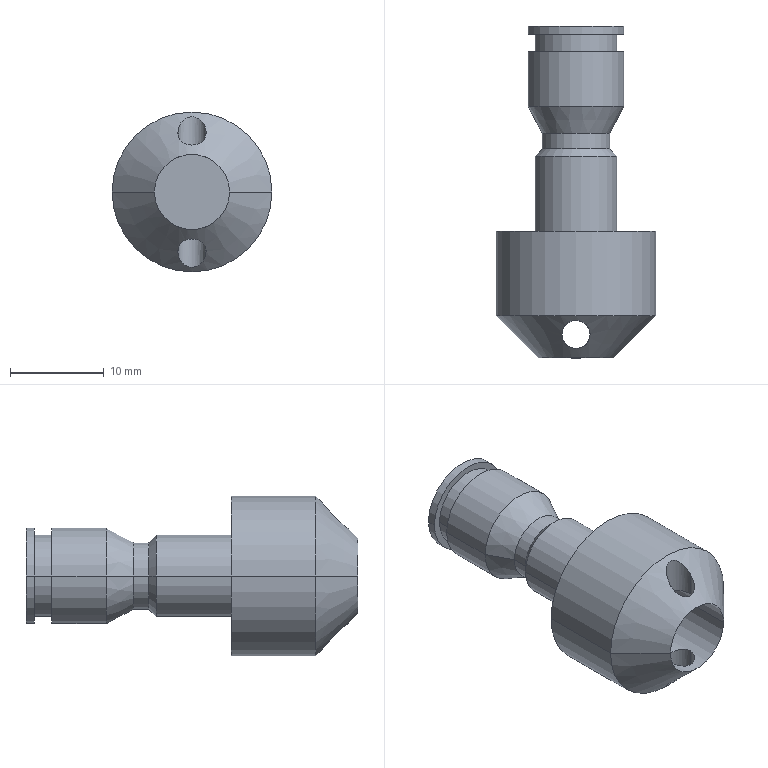Part | SolidWorks | features Cut 1, ICE 1, MirrorPattern 1, RevCut 1, Revolution 1 | 1 solid | 32 faces | box 17 x 35.31 x 17 mm | volume 3384 mm3 | cylinder 20 | cone 6 | plane 6 | commonest cylinder face diameters 3 x4 8.682 x4 10.203 x4 5.5 x2 7.161 x2 8 x2
STEP:
#1=CARTESIAN_POINT('',(-1.5,-17.445,6.325));
#2=VERTEX_POINT('',#1);
#3=CARTESIAN_POINT('',(1.5,-17.445,6.325));
#4=VERTEX_POINT('',#3);
#5=CARTESIAN_POINT('',(-1.5,-17.445,6.325));
#6=CARTESIAN_POINT('',(-1.5,-17.274,6.501));
#7=CARTESIAN_POINT('',(-1.472,-17.107,6.679));
#8=CARTESIAN_POINT('',(-1.356,-16.781,7.035));
#9=CARTESIAN_POINT('',(-1.271,-16.627,7.208));
#10=CARTESIAN_POINT('',(-1.033,-16.342,7.534));
#11=CARTESIAN_POINT('',(-0.8798,-16.211,7.687));
#12=CARTESIAN_POINT('',(-0.5873,-16.06,7.863));
#13=CARTESIAN_POINT('',(-0.4808,-16.019,7.912));
#14=CARTESIAN_POINT('',(-0.2477,-15.961,7.981));
#15=CARTESIAN_POINT('',(-0.1246,-15.945,8.));
#16=CARTESIAN_POINT('',(0.1245,-15.945,8.));
#17=CARTESIAN_POINT('',(0.248,-15.961,7.981));
#18=CARTESIAN_POINT('',(0.4799,-16.019,7.913));
#19=CARTESIAN_POINT('',(0.5882,-16.061,7.863));
#20=CARTESIAN_POINT('',(0.8792,-16.21,7.687));
#21=CARTESIAN_POINT('',(1.033,-16.342,7.534));
#22=CARTESIAN_POINT('',(1.27,-16.626,7.21));
#23=CARTESIAN_POINT('',(1.357,-16.782,7.034));
#24=CARTESIAN_POINT('',(1.471,-17.105,6.681));
#25=CARTESIAN_POINT('',(1.5,-17.272,6.502));
#26=CARTESIAN_POINT('',(1.5,-17.445,6.325));
#27=B_SPLINE_CURVE_WITH_KNOTS('',3,(#5,#6,#7,#8,#9,#10,#11,#12,#13,#14,#15,#16,#17,#18,#19,#20,#21,#22,#23,#24,#25,#26),.UNSPECIFIED.,.F.,.F.,(4,2,2,2,2,2,2,2,2,2,4),(0.0021,0.002839,0.003577,0.004316,0.004685,0.005054,0.005424,0.005793,0.006531,0.00727,0.008009),.UNSPECIFIED.);
#28=EDGE_CURVE('',#2,#4,#27,.T.);
#29=ORIENTED_EDGE('',*,*,#28,.F.);
#30=CARTESIAN_POINT('',(-1.5,-17.445,3.708));
#31=VERTEX_POINT('',#30);
#32=CARTESIAN_POINT('',(-1.5,-17.445,3.483));
#33=DIRECTION('',(0.,0.,-1.));
#34=VECTOR('',#33,1000.);
#35=LINE('',#32,#34);
#36=EDGE_CURVE('',#2,#31,#35,.T.);
#37=ORIENTED_EDGE('',*,*,#36,.T.);
#38=CARTESIAN_POINT('',(1.5,-17.445,3.708));
#39=VERTEX_POINT('',#38);
#40=CARTESIAN_POINT('',(-1.5,-17.445,3.708));
#41=CARTESIAN_POINT('',(-1.5,-17.248,3.708));
#42=CARTESIAN_POINT('',(-1.46,-17.049,3.725));
#43=CARTESIAN_POINT('',(-1.347,-16.777,3.767));
#44=CARTESIAN_POINT('',(-1.3,-16.69,3.783));
#45=CARTESIAN_POINT('',(-1.191,-16.529,3.819));
#46=CARTESIAN_POINT('',(-1.13,-16.453,3.838));
#47=CARTESIAN_POINT('',(-0.9215,-16.245,3.895));
#48=CARTESIAN_POINT('',(-0.7581,-16.136,3.932));
#49=CARTESIAN_POINT('',(-0.4854,-16.022,3.971));
#50=CARTESIAN_POINT('',(-0.3917,-15.994,3.982));
#51=CARTESIAN_POINT('',(-0.1986,-15.955,3.996));
#52=CARTESIAN_POINT('',(-0.09814,-15.945,4.));
#53=CARTESIAN_POINT('',(0.1984,-15.945,4.));
#54=CARTESIAN_POINT('',(0.3972,-15.985,3.984));
#55=CARTESIAN_POINT('',(0.7586,-16.136,3.932));
#56=CARTESIAN_POINT('',(0.924,-16.248,3.894));
#57=CARTESIAN_POINT('',(1.13,-16.454,3.838));
#58=CARTESIAN_POINT('',(1.193,-16.53,3.818));
#59=CARTESIAN_POINT('',(1.301,-16.692,3.783));
#60=CARTESIAN_POINT('',(1.347,-16.778,3.767));
#61=CARTESIAN_POINT('',(1.461,-17.051,3.725));
#62=CARTESIAN_POINT('',(1.5,-17.245,3.708));
#63=CARTESIAN_POINT('',(1.5,-17.445,3.708));
#64=B_SPLINE_CURVE_WITH_KNOTS('',3,(#40,#41,#42,#43,#44,#45,#46,#47,#48,#49,#50,#51,#52,#53,#54,#55,#56,#57,#58,#59,#60,#61,#62,#63),.UNSPECIFIED.,.F.,.F.,(4,2,2,2,2,2,2,2,2,2,2,4),(0.004733,0.005325,0.00562,0.005916,0.006508,0.006803,0.007099,0.007691,0.008282,0.008578,0.008874,0.009465),.UNSPECIFIED.);
#65=EDGE_CURVE('',#31,#39,#64,.T.);
#66=ORIENTED_EDGE('',*,*,#65,.T.);
#67=CARTESIAN_POINT('',(1.5,-17.445,3.483));
#68=DIRECTION('',(0.,0.,-1.));
#69=VECTOR('',#68,1000.);
#70=LINE('',#67,#69);
#71=EDGE_CURVE('',#4,#39,#70,.T.);
#72=ORIENTED_EDGE('',*,*,#71,.F.);
#73=EDGE_LOOP('',(#29,#37,#66,#72));
#74=FACE_OUTER_BOUND('',#73,.T.);
#75=CARTESIAN_POINT('',(0.,-17.445,3.483));
#76=DIRECTION('',(0.,0.,-1.));
#77=DIRECTION('',(1.,0.,0.));
#78=AXIS2_PLACEMENT_3D('',#75,#76,#77);
#79=CYLINDRICAL_SURFACE('',#78,1.5);
#80=ADVANCED_FACE('',(#74),#79,.F.);
#81=CARTESIAN_POINT('',(-1.5,-17.445,-6.325));
#82=VERTEX_POINT('',#81);
#83=CARTESIAN_POINT('',(1.5,-17.445,-6.325));
#84=VERTEX_POINT('',#83);
#85=CARTESIAN_POINT('',(-1.5,-17.445,-6.325));
#86=CARTESIAN_POINT('',(-1.5,-17.607,-6.158));
#87=CARTESIAN_POINT('',(-1.474,-17.773,-5.994));
#88=CARTESIAN_POINT('',(-1.362,-18.098,-5.687));
#89=CARTESIAN_POINT('',(-1.273,-18.261,-5.54));
#90=CARTESIAN_POINT('',(-1.024,-18.558,-5.29));
#91=CARTESIAN_POINT('',(-0.8599,-18.694,-5.184));
#92=CARTESIAN_POINT('',(-0.5617,-18.84,-5.075));
#93=CARTESIAN_POINT('',(-0.4548,-18.879,-5.047));
#94=CARTESIAN_POINT('',(-0.2332,-18.931,-5.01));
#95=CARTESIAN_POINT('',(-0.1157,-18.945,-5.));
#96=CARTESIAN_POINT('',(0.1157,-18.945,-5.));
#97=CARTESIAN_POINT('',(0.2323,-18.931,-5.009));
#98=CARTESIAN_POINT('',(0.4559,-18.879,-5.047));
#99=CARTESIAN_POINT('',(0.562,-18.84,-5.075));
#100=CARTESIAN_POINT('',(0.8615,-18.693,-5.184));
#101=CARTESIAN_POINT('',(1.025,-18.557,-5.291));
#102=CARTESIAN_POINT('',(1.274,-18.26,-5.541));
#103=CARTESIAN_POINT('',(1.362,-18.096,-5.688));
#104=CARTESIAN_POINT('',(1.474,-17.772,-5.995));
#105=CARTESIAN_POINT('',(1.5,-17.606,-6.159));
#106=CARTESIAN_POINT('',(1.5,-17.445,-6.325));
#107=B_SPLINE_CURVE_WITH_KNOTS('',3,(#85,#86,#87,#88,#89,#90,#91,#92,#93,#94,#95,#96,#97,#98,#99,#100,#101,#102,#103,#104,#105,#106),.UNSPECIFIED.,.F.,.F.,(4,2,2,2,2,2,2,2,2,2,4),(0.01111,0.0118,0.01249,0.01319,0.01353,0.01388,0.01422,0.01457,0.01526,0.01595,0.01664),.UNSPECIFIED.);
#108=EDGE_CURVE('',#82,#84,#107,.T.);
#109=ORIENTED_EDGE('',*,*,#108,.F.);
#110=CARTESIAN_POINT('',(-1.5,-17.445,-3.708));
#111=VERTEX_POINT('',#110);
#112=CARTESIAN_POINT('',(-1.5,-17.445,-3.483));
#113=DIRECTION('',(0.,0.,1.));
#114=VECTOR('',#113,1000.);
#115=LINE('',#112,#114);
#116=EDGE_CURVE('',#82,#111,#115,.T.);
#117=ORIENTED_EDGE('',*,*,#116,.T.);
#118=CARTESIAN_POINT('',(1.5,-17.445,-3.708));
#119=VERTEX_POINT('',#118);
#120=CARTESIAN_POINT('',(-1.5,-17.445,-3.708));
#121=CARTESIAN_POINT('',(-1.5,-17.642,-3.708));
#122=CARTESIAN_POINT('',(-1.46,-17.841,-3.725));
#123=CARTESIAN_POINT('',(-1.347,-18.113,-3.767));
#124=CARTESIAN_POINT('',(-1.3,-18.2,-3.783));
#125=CARTESIAN_POINT('',(-1.191,-18.362,-3.819));
#126=CARTESIAN_POINT('',(-1.13,-18.437,-3.838));
#127=CARTESIAN_POINT('',(-0.9215,-18.645,-3.895));
#128=CARTESIAN_POINT('',(-0.7581,-18.754,-3.932));
#129=CARTESIAN_POINT('',(-0.4854,-18.868,-3.971));
#130=CARTESIAN_POINT('',(-0.3917,-18.896,-3.982));
#131=CARTESIAN_POINT('',(-0.1986,-18.935,-3.996));
#132=CARTESIAN_POINT('',(-0.09814,-18.945,-4.));
#133=CARTESIAN_POINT('',(0.1984,-18.945,-4.));
#134=CARTESIAN_POINT('',(0.3972,-18.905,-3.984));
#135=CARTESIAN_POINT('',(0.7586,-18.754,-3.932));
#136=CARTESIAN_POINT('',(0.924,-18.643,-3.894));
#137=CARTESIAN_POINT('',(1.13,-18.436,-3.838));
#138=CARTESIAN_POINT('',(1.193,-18.36,-3.818));
#139=CARTESIAN_POINT('',(1.301,-18.198,-3.783));
#140=CARTESIAN_POINT('',(1.347,-18.112,-3.767));
#141=CARTESIAN_POINT('',(1.461,-17.839,-3.725));
#142=CARTESIAN_POINT('',(1.5,-17.645,-3.708));
#143=CARTESIAN_POINT('',(1.5,-17.445,-3.708));
#144=B_SPLINE_CURVE_WITH_KNOTS('',3,(#120,#121,#122,#123,#124,#125,#126,#127,#128,#129,#130,#131,#132,#133,#134,#135,#136,#137,#138,#139,#140,#141,#142,#143),.UNSPECIFIED.,.F.,.F.,(4,2,2,2,2,2,2,2,2,2,2,4),(0.004733,0.005325,0.00562,0.005916,0.006508,0.006803,0.007099,0.007691,0.008282,0.008578,0.008874,0.009465),.UNSPECIFIED.);
#145=EDGE_CURVE('',#111,#119,#144,.T.);
#146=ORIENTED_EDGE('',*,*,#145,.T.);
#147=CARTESIAN_POINT('',(1.5,-17.445,-3.483));
#148=DIRECTION('',(0.,0.,1.));
#149=VECTOR('',#148,1000.);
#150=LINE('',#147,#149);
#151=EDGE_CURVE('',#84,#119,#150,.T.);
#152=ORIENTED_EDGE('',*,*,#151,.F.);
#153=EDGE_LOOP('',(#109,#117,#146,#152));
#154=FACE_OUTER_BOUND('',#153,.T.);
#155=CARTESIAN_POINT('',(0.,-17.445,-3.483));
#156=DIRECTION('',(0.,0.,1.));
#157=DIRECTION('',(1.,0.,0.));
#158=AXIS2_PLACEMENT_3D('',#155,#156,#157);
#159=CYLINDRICAL_SURFACE('',#158,1.5);
#160=ADVANCED_FACE('',(#154),#159,.F.);
#161=CARTESIAN_POINT('',(2.75,11.365,0.));
#162=VERTEX_POINT('',#161);
#163=CARTESIAN_POINT('',(-2.75,11.365,0.));
#164=VERTEX_POINT('',#163);
#165=CARTESIAN_POINT('',(0.,11.365,0.));
#166=DIRECTION('',(0.,1.,0.));
#167=DIRECTION('',(-1.,0.,0.));
#168=AXIS2_PLACEMENT_3D('',#165,#166,#167);
#169=CIRCLE('',#168,2.75);
#170=EDGE_CURVE('',#162,#164,#169,.T.);
#171=ORIENTED_EDGE('',*,*,#170,.F.);
#172=CARTESIAN_POINT('',(2.75,15.365,0.));
#173=VERTEX_POINT('',#172);
#174=CARTESIAN_POINT('',(2.75,11.365,0.));
#175=DIRECTION('',(0.,1.,0.));
#176=VECTOR('',#175,1000.);
#177=LINE('',#174,#176);
#178=EDGE_CURVE('',#162,#173,#177,.T.);
#179=ORIENTED_EDGE('',*,*,#178,.T.);
#180=CARTESIAN_POINT('',(-2.75,15.365,0.));
#181=VERTEX_POINT('',#180);
#182=CARTESIAN_POINT('',(0.,15.365,0.));
#183=DIRECTION('',(0.,1.,0.));
#184=DIRECTION('',(-1.,0.,0.));
#185=AXIS2_PLACEMENT_3D('',#182,#183,#184);
#186=CIRCLE('',#185,2.75);
#187=EDGE_CURVE('',#173,#181,#186,.T.);
#188=ORIENTED_EDGE('',*,*,#187,.T.);
#189=CARTESIAN_POINT('',(-2.75,11.365,0.));
#190=DIRECTION('',(0.,1.,0.));
#191=VECTOR('',#190,1000.);
#192=LINE('',#189,#191);
#193=EDGE_CURVE('',#164,#181,#192,.T.);
#194=ORIENTED_EDGE('',*,*,#193,.F.);
#195=EDGE_LOOP('',(#171,#179,#188,#194));
#196=FACE_OUTER_BOUND('',#195,.T.);
#197=CARTESIAN_POINT('',(0.,11.365,0.));
#198=DIRECTION('',(0.,1.,0.));
#199=DIRECTION('',(-1.,0.,0.));
#200=AXIS2_PLACEMENT_3D('',#197,#198,#199);
#201=CYLINDRICAL_SURFACE('',#200,2.75);
#202=ADVANCED_FACE('',(#196),#201,.F.);
#203=CARTESIAN_POINT('',(-8.5,-15.445,0.));
#204=VERTEX_POINT('',#203);
#205=CARTESIAN_POINT('',(8.5,-15.445,0.));
#206=VERTEX_POINT('',#205);
#207=CARTESIAN_POINT('',(0.,-15.445,0.));
#208=DIRECTION('',(0.,1.,0.));
#209=DIRECTION('',(-1.,0.,0.));
#210=AXIS2_PLACEMENT_3D('',#207,#208,#209);
#211=CIRCLE('',#210,8.5);
#212=EDGE_CURVE('',#204,#206,#211,.T.);
#213=ORIENTED_EDGE('',*,*,#212,.T.);
#214=CARTESIAN_POINT('',(8.5,-6.487,0.));
#215=VERTEX_POINT('',#214);
#216=CARTESIAN_POINT('',(8.5,12.634,0.));
#217=DIRECTION('',(0.,1.,0.));
#218=VECTOR('',#217,1000.);
#219=LINE('',#216,#218);
#220=EDGE_CURVE('',#206,#215,#219,.T.);
#221=ORIENTED_EDGE('',*,*,#220,.T.);
#222=CARTESIAN_POINT('',(-8.5,-6.487,0.));
#223=VERTEX_POINT('',#222);
#224=CARTESIAN_POINT('',(0.,-6.487,0.));
#225=DIRECTION('',(0.,1.,0.));
#226=DIRECTION('',(-1.,0.,0.));
#227=AXIS2_PLACEMENT_3D('',#224,#225,#226);
#228=CIRCLE('',#227,8.5);
#229=EDGE_CURVE('',#223,#215,#228,.T.);
#230=ORIENTED_EDGE('',*,*,#229,.F.);
#231=CARTESIAN_POINT('',(-8.5,12.634,0.));
#232=DIRECTION('',(0.,1.,0.));
#233=VECTOR('',#232,1000.);
#234=LINE('',#231,#233);
#235=EDGE_CURVE('',#204,#223,#234,.T.);
#236=ORIENTED_EDGE('',*,*,#235,.F.);
#237=EDGE_LOOP('',(#213,#221,#230,#236));
#238=FACE_OUTER_BOUND('',#237,.T.);
#239=CARTESIAN_POINT('',(0.,12.634,0.));
#240=DIRECTION('',(0.,1.,0.));
#241=DIRECTION('',(-1.,0.,0.));
#242=AXIS2_PLACEMENT_3D('',#239,#240,#241);
#243=CYLINDRICAL_SURFACE('',#242,8.5);
#244=ADVANCED_FACE('',(#238),#243,.T.);
#245=CARTESIAN_POINT('',(-4.341,-6.487,0.));
#246=VERTEX_POINT('',#245);
#247=CARTESIAN_POINT('',(4.341,-6.487,0.));
#248=VERTEX_POINT('',#247);
#249=CARTESIAN_POINT('',(0.,-6.487,0.));
#250=DIRECTION('',(0.,1.,0.));
#251=DIRECTION('',(-1.,0.,0.));
#252=AXIS2_PLACEMENT_3D('',#249,#250,#251);
#253=CIRCLE('',#252,4.341);
#254=EDGE_CURVE('',#246,#248,#253,.T.);
#255=ORIENTED_EDGE('',*,*,#254,.T.);
#256=CARTESIAN_POINT('',(4.341,1.533,0.));
#257=VERTEX_POINT('',#256);
#258=CARTESIAN_POINT('',(4.341,12.634,0.));
#259=DIRECTION('',(0.,1.,0.));
#260=VECTOR('',#259,1000.);
#261=LINE('',#258,#260);
#262=EDGE_CURVE('',#248,#257,#261,.T.);
#263=ORIENTED_EDGE('',*,*,#262,.T.);
#264=CARTESIAN_POINT('',(-4.341,1.533,0.));
#265=VERTEX_POINT('',#264);
#266=CARTESIAN_POINT('',(0.,1.533,0.));
#267=DIRECTION('',(0.,1.,0.));
#268=DIRECTION('',(-1.,0.,0.));
#269=AXIS2_PLACEMENT_3D('',#266,#267,#268);
#270=CIRCLE('',#269,4.341);
#271=EDGE_CURVE('',#265,#257,#270,.T.);
#272=ORIENTED_EDGE('',*,*,#271,.F.);
#273=CARTESIAN_POINT('',(-4.341,12.634,0.));
#274=DIRECTION('',(0.,1.,0.));
#275=VECTOR('',#274,1000.);
#276=LINE('',#273,#275);
#277=EDGE_CURVE('',#246,#265,#276,.T.);
#278=ORIENTED_EDGE('',*,*,#277,.F.);
#279=EDGE_LOOP('',(#255,#263,#272,#278));
#280=FACE_OUTER_BOUND('',#279,.T.);
#281=CARTESIAN_POINT('',(0.,12.634,0.));
#282=DIRECTION('',(0.,1.,0.));
#283=DIRECTION('',(-1.,0.,0.));
#284=AXIS2_PLACEMENT_3D('',#281,#282,#283);
#285=CYLINDRICAL_SURFACE('',#284,4.341);
#286=ADVANCED_FACE('',(#280),#285,.T.);
#287=CARTESIAN_POINT('',(-3.581,2.293,0.));
#288=VERTEX_POINT('',#287);
#289=CARTESIAN_POINT('',(3.581,2.293,0.));
#290=VERTEX_POINT('',#289);
#291=CARTESIAN_POINT('',(0.,2.293,0.));
#292=DIRECTION('',(0.,1.,0.));
#293=DIRECTION('',(-1.,0.,0.));
#294=AXIS2_PLACEMENT_3D('',#291,#292,#293);
#295=CIRCLE('',#294,3.581);
#296=EDGE_CURVE('',#288,#290,#295,.T.);
#297=ORIENTED_EDGE('',*,*,#296,.F.);
#298=CARTESIAN_POINT('',(-3.581,2.293,0.));
#299=DIRECTION('',(-0.7071,-0.7071,0.));
#300=VECTOR('',#299,1000.);
#301=LINE('',#298,#300);
#302=EDGE_CURVE('',#288,#265,#301,.T.);
#303=ORIENTED_EDGE('',*,*,#302,.T.);
#304=ORIENTED_EDGE('',*,*,#271,.T.);
#305=CARTESIAN_POINT('',(3.581,2.293,0.));
#306=DIRECTION('',(0.7071,-0.7071,0.));
#307=VECTOR('',#306,1000.);
#308=LINE('',#305,#307);
#309=EDGE_CURVE('',#290,#257,#308,.T.);
#310=ORIENTED_EDGE('',*,*,#309,.F.);
#311=EDGE_LOOP('',(#297,#303,#304,#310));
#312=FACE_OUTER_BOUND('',#311,.T.);
#313=CARTESIAN_POINT('',(0.,2.293,0.));
#314=DIRECTION('',(0.,-1.,0.));
#315=DIRECTION('',(1.,0.,0.));
#316=AXIS2_PLACEMENT_3D('',#313,#314,#315);
#317=CONICAL_SURFACE('',#316,3.581,0.7854);
#318=ADVANCED_FACE('',(#312),#317,.T.);
#319=ORIENTED_EDGE('',*,*,#296,.T.);
#320=CARTESIAN_POINT('',(3.581,3.948,0.));
#321=VERTEX_POINT('',#320);
#322=CARTESIAN_POINT('',(3.581,12.634,0.));
#323=DIRECTION('',(0.,1.,0.));
#324=VECTOR('',#323,1000.);
#325=LINE('',#322,#324);
#326=EDGE_CURVE('',#290,#321,#325,.T.);
#327=ORIENTED_EDGE('',*,*,#326,.T.);
#328=CARTESIAN_POINT('',(-3.581,3.948,0.));
#329=VERTEX_POINT('',#328);
#330=CARTESIAN_POINT('',(0.,3.948,0.));
#331=DIRECTION('',(0.,1.,0.));
#332=DIRECTION('',(-1.,0.,0.));
#333=AXIS2_PLACEMENT_3D('',#330,#331,#332);
#334=CIRCLE('',#333,3.581);
#335=EDGE_CURVE('',#329,#321,#334,.T.);
#336=ORIENTED_EDGE('',*,*,#335,.F.);
#337=CARTESIAN_POINT('',(-3.581,12.634,0.));
#338=DIRECTION('',(0.,1.,0.));
#339=VECTOR('',#338,1000.);
#340=LINE('',#337,#339);
#341=EDGE_CURVE('',#288,#329,#340,.T.);
#342=ORIENTED_EDGE('',*,*,#341,.F.);
#343=EDGE_LOOP('',(#319,#327,#336,#342));
#344=FACE_OUTER_BOUND('',#343,.T.);
#345=CARTESIAN_POINT('',(0.,12.634,0.));
#346=DIRECTION('',(0.,1.,0.));
#347=DIRECTION('',(-1.,0.,0.));
#348=AXIS2_PLACEMENT_3D('',#345,#346,#347);
#349=CYLINDRICAL_SURFACE('',#348,3.581);
#350=ADVANCED_FACE('',(#344),#349,.T.);
#351=ORIENTED_EDGE('',*,*,#335,.T.);
#352=CARTESIAN_POINT('',(5.102,6.827,0.));
#353=VERTEX_POINT('',#352);
#354=CARTESIAN_POINT('',(5.102,6.827,0.));
#355=DIRECTION('',(0.4672,0.8842,0.));
#356=VECTOR('',#355,1000.);
#357=LINE('',#354,#356);
#358=EDGE_CURVE('',#321,#353,#357,.T.);
#359=ORIENTED_EDGE('',*,*,#358,.T.);
#360=CARTESIAN_POINT('',(-5.102,6.827,0.));
#361=VERTEX_POINT('',#360);
#362=CARTESIAN_POINT('',(0.,6.827,0.));
#363=DIRECTION('',(0.,1.,0.));
#364=DIRECTION('',(-1.,0.,0.));
#365=AXIS2_PLACEMENT_3D('',#362,#363,#364);
#366=CIRCLE('',#365,5.102);
#367=EDGE_CURVE('',#361,#353,#366,.T.);
#368=ORIENTED_EDGE('',*,*,#367,.F.);
#369=CARTESIAN_POINT('',(-5.102,6.827,0.));
#370=DIRECTION('',(-0.4672,0.8842,0.));
#371=VECTOR('',#370,1000.);
#372=LINE('',#369,#371);
#373=EDGE_CURVE('',#329,#361,#372,.T.);
#374=ORIENTED_EDGE('',*,*,#373,.F.);
#375=EDGE_LOOP('',(#351,#359,#368,#374));
#376=FACE_OUTER_BOUND('',#375,.T.);
#377=CARTESIAN_POINT('',(0.,6.827,0.));
#378=DIRECTION('',(0.,1.,0.));
#379=DIRECTION('',(-1.,0.,0.));
#380=AXIS2_PLACEMENT_3D('',#377,#378,#379);
#381=CONICAL_SURFACE('',#380,5.102,0.4861);
#382=ADVANCED_FACE('',(#376),#381,.T.);
#383=ORIENTED_EDGE('',*,*,#367,.T.);
#384=CARTESIAN_POINT('',(5.102,12.634,0.));
#385=VERTEX_POINT('',#384);
#386=CARTESIAN_POINT('',(5.102,12.634,0.));
#387=DIRECTION('',(0.,1.,0.));
#388=VECTOR('',#387,1000.);
#389=LINE('',#386,#388);
#390=EDGE_CURVE('',#353,#385,#389,.T.);
#391=ORIENTED_EDGE('',*,*,#390,.T.);
#392=CARTESIAN_POINT('',(-5.102,12.634,0.));
#393=VERTEX_POINT('',#392);
#394=CARTESIAN_POINT('',(0.,12.634,0.));
#395=DIRECTION('',(0.,1.,0.));
#396=DIRECTION('',(-1.,0.,0.));
#397=AXIS2_PLACEMENT_3D('',#394,#395,#396);
#398=CIRCLE('',#397,5.102);
#399=EDGE_CURVE('',#393,#385,#398,.T.);
#400=ORIENTED_EDGE('',*,*,#399,.F.);
#401=CARTESIAN_POINT('',(-5.102,12.634,0.));
#402=DIRECTION('',(0.,1.,0.));
#403=VECTOR('',#402,1000.);
#404=LINE('',#401,#403);
#405=EDGE_CURVE('',#361,#393,#404,.T.);
#406=ORIENTED_EDGE('',*,*,#405,.F.);
#407=EDGE_LOOP('',(#383,#391,#400,#406));
#408=FACE_OUTER_BOUND('',#407,.T.);
#409=CARTESIAN_POINT('',(0.,12.634,0.));
#410=DIRECTION('',(0.,1.,0.));
#411=DIRECTION('',(-1.,0.,0.));
#412=AXIS2_PLACEMENT_3D('',#409,#410,#411);
#413=CYLINDRICAL_SURFACE('',#412,5.102);
#414=ADVANCED_FACE('',(#408),#413,.T.);
#415=CARTESIAN_POINT('',(-4.341,12.634,0.));
#416=VERTEX_POINT('',#415);
#417=CARTESIAN_POINT('',(4.341,12.634,0.));
#418=VERTEX_POINT('',#417);
#419=CARTESIAN_POINT('',(0.,12.634,0.));
#420=DIRECTION('',(0.,1.,0.));
#421=DIRECTION('',(-1.,0.,0.));
#422=AXIS2_PLACEMENT_3D('',#419,#420,#421);
#423=CIRCLE('',#422,4.341);
#424=EDGE_CURVE('',#416,#418,#423,.T.);
#425=ORIENTED_EDGE('',*,*,#424,.T.);
#426=CARTESIAN_POINT('',(4.341,14.471,0.));
#427=VERTEX_POINT('',#426);
#428=CARTESIAN_POINT('',(4.341,12.634,0.));
#429=DIRECTION('',(0.,1.,0.));
#430=VECTOR('',#429,1000.);
#431=LINE('',#428,#430);
#432=EDGE_CURVE('',#418,#427,#431,.T.);
#433=ORIENTED_EDGE('',*,*,#432,.T.);
#434=CARTESIAN_POINT('',(-4.341,14.471,0.));
#435=VERTEX_POINT('',#434);
#436=CARTESIAN_POINT('',(0.,14.471,0.));
#437=DIRECTION('',(0.,1.,0.));
#438=DIRECTION('',(-1.,0.,0.));
#439=AXIS2_PLACEMENT_3D('',#436,#437,#438);
#440=CIRCLE('',#439,4.341);
#441=EDGE_CURVE('',#435,#427,#440,.T.);
#442=ORIENTED_EDGE('',*,*,#441,.F.);
#443=CARTESIAN_POINT('',(-4.341,12.634,0.));
#444=DIRECTION('',(0.,1.,0.));
#445=VECTOR('',#444,1000.);
#446=LINE('',#443,#445);
#447=EDGE_CURVE('',#416,#435,#446,.T.);
#448=ORIENTED_EDGE('',*,*,#447,.F.);
#449=EDGE_LOOP('',(#425,#433,#442,#448));
#450=FACE_OUTER_BOUND('',#449,.T.);
#451=CARTESIAN_POINT('',(0.,12.634,0.));
#452=DIRECTION('',(0.,1.,0.));
#453=DIRECTION('',(-1.,0.,0.));
#454=AXIS2_PLACEMENT_3D('',#451,#452,#453);
#455=CYLINDRICAL_SURFACE('',#454,4.341);
#456=ADVANCED_FACE('',(#450),#455,.T.);
#457=CARTESIAN_POINT('',(-5.102,14.471,0.));
#458=VERTEX_POINT('',#457);
#459=CARTESIAN_POINT('',(5.102,14.471,0.));
#460=VERTEX_POINT('',#459);
#461=CARTESIAN_POINT('',(0.,14.471,0.));
#462=DIRECTION('',(0.,1.,0.));
#463=DIRECTION('',(-1.,0.,0.));
#464=AXIS2_PLACEMENT_3D('',#461,#462,#463);
#465=CIRCLE('',#464,5.102);
#466=EDGE_CURVE('',#458,#460,#465,.T.);
#467=ORIENTED_EDGE('',*,*,#466,.T.);
#468=CARTESIAN_POINT('',(5.102,15.365,0.));
#469=VERTEX_POINT('',#468);
#470=CARTESIAN_POINT('',(5.102,12.634,0.));
#471=DIRECTION('',(0.,1.,0.));
#472=VECTOR('',#471,1000.);
#473=LINE('',#470,#472);
#474=EDGE_CURVE('',#460,#469,#473,.T.);
#475=ORIENTED_EDGE('',*,*,#474,.T.);
#476=CARTESIAN_POINT('',(-5.102,15.365,0.));
#477=VERTEX_POINT('',#476);
#478=CARTESIAN_POINT('',(0.,15.365,0.));
#479=DIRECTION('',(0.,1.,0.));
#480=DIRECTION('',(-1.,0.,0.));
#481=AXIS2_PLACEMENT_3D('',#478,#479,#480);
#482=CIRCLE('',#481,5.102);
#483=EDGE_CURVE('',#477,#469,#482,.T.);
#484=ORIENTED_EDGE('',*,*,#483,.F.);
#485=CARTESIAN_POINT('',(-5.102,12.634,0.));
#486=DIRECTION('',(0.,1.,0.));
#487=VECTOR('',#486,1000.);
#488=LINE('',#485,#487);
#489=EDGE_CURVE('',#458,#477,#488,.T.);
#490=ORIENTED_EDGE('',*,*,#489,.F.);
#491=EDGE_LOOP('',(#467,#475,#484,#490));
#492=FACE_OUTER_BOUND('',#491,.T.);
#493=CARTESIAN_POINT('',(0.,12.634,0.));
#494=DIRECTION('',(0.,1.,0.));
#495=DIRECTION('',(-1.,0.,0.));
#496=AXIS2_PLACEMENT_3D('',#493,#494,#495);
#497=CYLINDRICAL_SURFACE('',#496,5.102);
#498=ADVANCED_FACE('',(#492),#497,.T.);
#499=CARTESIAN_POINT('',(1.5,-17.445,-3.708));
#500=CARTESIAN_POINT('',(1.5,-17.345,-3.708));
#501=CARTESIAN_POINT('',(1.49,-17.247,-3.712));
#502=CARTESIAN_POINT('',(1.451,-17.054,-3.727));
#503=CARTESIAN_POINT('',(1.422,-16.958,-3.739));
#504=CARTESIAN_POINT('',(1.309,-16.686,-3.781));
#505=CARTESIAN_POINT('',(1.198,-16.521,-3.819));
#506=CARTESIAN_POINT('',(0.9235,-16.247,-3.895));
#507=CARTESIAN_POINT('',(0.7577,-16.136,-3.932));
#508=CARTESIAN_POINT('',(0.4873,-16.023,-3.971));
#509=CARTESIAN_POINT('',(0.3918,-15.994,-3.982));
#510=CARTESIAN_POINT('',(0.1976,-15.955,-3.996));
#511=CARTESIAN_POINT('',(0.09965,-15.945,-4.));
#512=CARTESIAN_POINT('',(-0.09818,-15.945,-4.));
#513=CARTESIAN_POINT('',(-0.1986,-15.955,-3.996));
#514=CARTESIAN_POINT('',(-0.3918,-15.994,-3.982));
#515=CARTESIAN_POINT('',(-0.4859,-16.022,-3.971));
#516=CARTESIAN_POINT('',(-0.6688,-16.099,-3.945));
#517=CARTESIAN_POINT('',(-0.7549,-16.145,-3.929));
#518=CARTESIAN_POINT('',(-0.9165,-16.254,-3.894));
#519=CARTESIAN_POINT('',(-0.9928,-16.316,-3.875));
#520=CARTESIAN_POINT('',(-1.13,-16.454,-3.838));
#521=CARTESIAN_POINT('',(-1.192,-16.529,-3.819));
#522=CARTESIAN_POINT('',(-1.3,-16.691,-3.783));
#523=CARTESIAN_POINT('',(-1.347,-16.779,-3.766));
#524=CARTESIAN_POINT('',(-1.46,-17.049,-3.725));
#525=CARTESIAN_POINT('',(-1.5,-17.248,-3.708));
#526=CARTESIAN_POINT('',(-1.5,-17.445,-3.708));
#527=B_SPLINE_CURVE_WITH_KNOTS('',3,(#499,#500,#501,#502,#503,#504,#505,#506,#507,#508,#509,#510,#511,#512,#513,#514,#515,#516,#517,#518,#519,#520,#521,#522,#523,#524,#525,#526),.UNSPECIFIED.,.F.,.F.,(4,2,2,2,2,2,2,2,2,2,2,2,2,4),(0.,0.0002958,0.0005916,0.001183,0.001775,0.002071,0.002367,0.002662,0.002958,0.003254,0.00355,0.003846,0.004142,0.004733),.UNSPECIFIED.);
#528=EDGE_CURVE('',#119,#111,#527,.T.);
#529=ORIENTED_EDGE('',*,*,#528,.F.);
#530=ORIENTED_EDGE('',*,*,#145,.F.);
#531=EDGE_LOOP('',(#529,#530));
#532=FACE_BOUND('',#531,.T.);
#533=CARTESIAN_POINT('',(-4.,-9.945,0.));
#534=VERTEX_POINT('',#533);
#535=CARTESIAN_POINT('',(4.,-9.945,0.));
#536=VERTEX_POINT('',#535);
#537=CARTESIAN_POINT('',(0.,-9.945,0.));
#538=DIRECTION('',(0.,-1.,0.));
#539=DIRECTION('',(1.,0.,0.));
#540=AXIS2_PLACEMENT_3D('',#537,#538,#539);
#541=CIRCLE('',#540,4.);
#542=EDGE_CURVE('',#534,#536,#541,.T.);
#543=ORIENTED_EDGE('',*,*,#542,.F.);
#544=CARTESIAN_POINT('',(-4.,-19.945,0.));
#545=VERTEX_POINT('',#544);
#546=CARTESIAN_POINT('',(-4.,-9.945,0.));
#547=DIRECTION('',(0.,-1.,0.));
#548=VECTOR('',#547,1000.);
#549=LINE('',#546,#548);
#550=EDGE_CURVE('',#534,#545,#549,.T.);
#551=ORIENTED_EDGE('',*,*,#550,.T.);
#552=CARTESIAN_POINT('',(4.,-19.945,0.));
#553=VERTEX_POINT('',#552);
#554=CARTESIAN_POINT('',(0.,-19.945,0.));
#555=DIRECTION('',(0.,-1.,0.));
#556=DIRECTION('',(1.,0.,0.));
#557=AXIS2_PLACEMENT_3D('',#554,#555,#556);
#558=CIRCLE('',#557,4.);
#559=EDGE_CURVE('',#545,#553,#558,.T.);
#560=ORIENTED_EDGE('',*,*,#559,.T.);
#561=CARTESIAN_POINT('',(4.,-9.945,0.));
#562=DIRECTION('',(0.,-1.,0.));
#563=VECTOR('',#562,1000.);
#564=LINE('',#561,#563);
#565=EDGE_CURVE('',#536,#553,#564,.T.);
#566=ORIENTED_EDGE('',*,*,#565,.F.);
#567=EDGE_LOOP('',(#543,#551,#560,#566));
#568=FACE_OUTER_BOUND('',#567,.T.);
#569=CARTESIAN_POINT('',(0.,-9.945,0.));
#570=DIRECTION('',(0.,-1.,0.));
#571=DIRECTION('',(1.,0.,0.));
#572=AXIS2_PLACEMENT_3D('',#569,#570,#571);
#573=CYLINDRICAL_SURFACE('',#572,4.);
#574=ADVANCED_FACE('',(#532,#568),#573,.F.);
#575=CARTESIAN_POINT('',(1.5,-17.445,6.325));
#576=CARTESIAN_POINT('',(1.5,-17.607,6.158));
#577=CARTESIAN_POINT('',(1.475,-17.769,5.998));
#578=CARTESIAN_POINT('',(1.364,-18.093,5.691));
#579=CARTESIAN_POINT('',(1.276,-18.257,5.544));
#580=CARTESIAN_POINT('',(1.089,-18.481,5.355));
#581=CARTESIAN_POINT('',(1.016,-18.553,5.296));
#582=CARTESIAN_POINT('',(0.8537,-18.683,5.193));
#583=CARTESIAN_POINT('',(0.7633,-18.741,5.149));
#584=CARTESIAN_POINT('',(0.5635,-18.84,5.075));
#585=CARTESIAN_POINT('',(0.4581,-18.878,5.048));
#586=CARTESIAN_POINT('',(0.2356,-18.931,5.01));
#587=CARTESIAN_POINT('',(0.1179,-18.945,5.));
#588=CARTESIAN_POINT('',(-0.1137,-18.945,5.));
#589=CARTESIAN_POINT('',(-0.2314,-18.932,5.009));
#590=CARTESIAN_POINT('',(-0.4544,-18.879,5.047));
#591=CARTESIAN_POINT('',(-0.5611,-18.841,5.074));
#592=CARTESIAN_POINT('',(-0.7607,-18.743,5.147));
#593=CARTESIAN_POINT('',(-0.8505,-18.685,5.191));
#594=CARTESIAN_POINT('',(-1.013,-18.556,5.293));
#595=CARTESIAN_POINT('',(-1.086,-18.484,5.352));
#596=CARTESIAN_POINT('',(-1.274,-18.26,5.541));
#597=CARTESIAN_POINT('',(-1.362,-18.097,5.688));
#598=CARTESIAN_POINT('',(-1.474,-17.772,5.995));
#599=CARTESIAN_POINT('',(-1.5,-17.606,6.159));
#600=CARTESIAN_POINT('',(-1.5,-17.445,6.325));
#601=B_SPLINE_CURVE_WITH_KNOTS('',3,(#575,#576,#577,#578,#579,#580,#581,#582,#583,#584,#585,#586,#587,#588,#589,#590,#591,#592,#593,#594,#595,#596,#597,#598,#599,#600),.UNSPECIFIED.,.F.,.F.,(4,2,2,2,2,2,2,2,2,2,2,2,4),(0.008009,0.008701,0.009393,0.009739,0.01009,0.01043,0.01078,0.01112,0.01147,0.01182,0.01216,0.01285,0.01355),.UNSPECIFIED.);
#602=EDGE_CURVE('',#4,#2,#601,.T.);
#603=ORIENTED_EDGE('',*,*,#602,.T.);
#604=ORIENTED_EDGE('',*,*,#28,.T.);
#605=EDGE_LOOP('',(#603,#604));
#606=FACE_BOUND('',#605,.T.);
#607=CARTESIAN_POINT('',(0.,-19.945,0.));
#608=DIRECTION('',(0.,-1.,0.));
#609=DIRECTION('',(1.,0.,0.));
#610=AXIS2_PLACEMENT_3D('',#607,#608,#609);
#611=CIRCLE('',#610,4.);
#612=EDGE_CURVE('',#553,#545,#611,.T.);
#613=ORIENTED_EDGE('',*,*,#612,.F.);
#614=CARTESIAN_POINT('',(8.5,-15.445,0.));
#615=DIRECTION('',(0.7071,0.7071,0.));
#616=VECTOR('',#615,1000.);
#617=LINE('',#614,#616);
#618=EDGE_CURVE('',#553,#206,#617,.T.);
#619=ORIENTED_EDGE('',*,*,#618,.T.);
#620=ORIENTED_EDGE('',*,*,#212,.F.);
#621=CARTESIAN_POINT('',(-8.5,-15.445,0.));
#622=DIRECTION('',(-0.7071,0.7071,0.));
#623=VECTOR('',#622,1000.);
#624=LINE('',#621,#623);
#625=EDGE_CURVE('',#545,#204,#624,.T.);
#626=ORIENTED_EDGE('',*,*,#625,.F.);
#627=EDGE_LOOP('',(#613,#619,#620,#626));
#628=FACE_OUTER_BOUND('',#627,.T.);
#629=CARTESIAN_POINT('',(0.,-15.445,0.));
#630=DIRECTION('',(0.,1.,0.));
#631=DIRECTION('',(-1.,0.,0.));
#632=AXIS2_PLACEMENT_3D('',#629,#630,#631);
#633=CONICAL_SURFACE('',#632,8.5,0.7854);
#634=ADVANCED_FACE('',(#606,#628),#633,.T.);
#635=ORIENTED_EDGE('',*,*,#618,.F.);
#636=ORIENTED_EDGE('',*,*,#559,.F.);
#637=ORIENTED_EDGE('',*,*,#625,.T.);
#638=CARTESIAN_POINT('',(0.,-15.445,0.));
#639=DIRECTION('',(0.,1.,0.));
#640=DIRECTION('',(-1.,0.,0.));
#641=AXIS2_PLACEMENT_3D('',#638,#639,#640);
#642=CIRCLE('',#641,8.5);
#643=EDGE_CURVE('',#206,#204,#642,.T.);
#644=ORIENTED_EDGE('',*,*,#643,.F.);
#645=EDGE_LOOP('',(#635,#636,#637,#644));
#646=FACE_OUTER_BOUND('',#645,.T.);
#647=CARTESIAN_POINT('',(1.5,-17.445,-6.325));
#648=CARTESIAN_POINT('',(1.5,-17.274,-6.501));
#649=CARTESIAN_POINT('',(1.472,-17.107,-6.679));
#650=CARTESIAN_POINT('',(1.356,-16.781,-7.035));
#651=CARTESIAN_POINT('',(1.271,-16.627,-7.208));
#652=CARTESIAN_POINT('',(1.033,-16.342,-7.534));
#653=CARTESIAN_POINT('',(0.8797,-16.211,-7.687));
#654=CARTESIAN_POINT('',(0.5873,-16.06,-7.863));
#655=CARTESIAN_POINT('',(0.4808,-16.019,-7.912));
#656=CARTESIAN_POINT('',(0.2477,-15.961,-7.981));
#657=CARTESIAN_POINT('',(0.1246,-15.945,-8.));
#658=CARTESIAN_POINT('',(-0.1244,-15.945,-8.));
#659=CARTESIAN_POINT('',(-0.248,-15.961,-7.981));
#660=CARTESIAN_POINT('',(-0.4798,-16.019,-7.913));
#661=CARTESIAN_POINT('',(-0.5882,-16.061,-7.863));
#662=CARTESIAN_POINT('',(-0.8792,-16.21,-7.687));
#663=CARTESIAN_POINT('',(-1.033,-16.342,-7.534));
#664=CARTESIAN_POINT('',(-1.27,-16.626,-7.21));
#665=CARTESIAN_POINT('',(-1.357,-16.782,-7.034));
#666=CARTESIAN_POINT('',(-1.471,-17.105,-6.681));
#667=CARTESIAN_POINT('',(-1.5,-17.272,-6.503));
#668=CARTESIAN_POINT('',(-1.5,-17.445,-6.325));
#669=B_SPLINE_CURVE_WITH_KNOTS('',3,(#647,#648,#649,#650,#651,#652,#653,#654,#655,#656,#657,#658,#659,#660,#661,#662,#663,#664,#665,#666,#667,#668),.UNSPECIFIED.,.F.,.F.,(4,2,2,2,2,2,2,2,2,2,4),(0.005205,0.005944,0.006682,0.00742,0.007789,0.008158,0.008527,0.008896,0.009634,0.01037,0.01111),.UNSPECIFIED.);
#670=EDGE_CURVE('',#84,#82,#669,.T.);
#671=ORIENTED_EDGE('',*,*,#670,.T.);
#672=ORIENTED_EDGE('',*,*,#108,.T.);
#673=EDGE_LOOP('',(#671,#672));
#674=FACE_BOUND('',#673,.T.);
#675=CARTESIAN_POINT('',(0.,-15.445,0.));
#676=DIRECTION('',(0.,1.,0.));
#677=DIRECTION('',(-1.,0.,0.));
#678=AXIS2_PLACEMENT_3D('',#675,#676,#677);
#679=CONICAL_SURFACE('',#678,8.5,0.7854);
#680=ADVANCED_FACE('',(#646,#674),#679,.T.);
#681=ORIENTED_EDGE('',*,*,#550,.F.);
#682=CARTESIAN_POINT('',(0.,-9.945,0.));
#683=DIRECTION('',(0.,-1.,0.));
#684=DIRECTION('',(1.,0.,0.));
#685=AXIS2_PLACEMENT_3D('',#682,#683,#684);
#686=CIRCLE('',#685,4.);
#687=EDGE_CURVE('',#536,#534,#686,.T.);
#688=ORIENTED_EDGE('',*,*,#687,.F.);
#689=ORIENTED_EDGE('',*,*,#565,.T.);
#690=ORIENTED_EDGE('',*,*,#612,.T.);
#691=EDGE_LOOP('',(#681,#688,#689,#690));
#692=FACE_OUTER_BOUND('',#691,.T.);
#693=CARTESIAN_POINT('',(1.5,-17.445,3.708));
#694=CARTESIAN_POINT('',(1.5,-17.545,3.708));
#695=CARTESIAN_POINT('',(1.49,-17.643,3.712));
#696=CARTESIAN_POINT('',(1.451,-17.836,3.727));
#697=CARTESIAN_POINT('',(1.422,-17.932,3.739));
#698=CARTESIAN_POINT('',(1.309,-18.204,3.781));
#699=CARTESIAN_POINT('',(1.198,-18.369,3.819));
#700=CARTESIAN_POINT('',(0.9235,-18.643,3.895));
#701=CARTESIAN_POINT('',(0.7577,-18.754,3.932));
#702=CARTESIAN_POINT('',(0.4873,-18.867,3.971));
#703=CARTESIAN_POINT('',(0.3918,-18.896,3.982));
#704=CARTESIAN_POINT('',(0.1976,-18.935,3.996));
#705=CARTESIAN_POINT('',(0.09965,-18.945,4.));
#706=CARTESIAN_POINT('',(-0.09818,-18.945,4.));
#707=CARTESIAN_POINT('',(-0.1986,-18.935,3.996));
#708=CARTESIAN_POINT('',(-0.3918,-18.896,3.982));
#709=CARTESIAN_POINT('',(-0.4859,-18.868,3.971));
#710=CARTESIAN_POINT('',(-0.6688,-18.791,3.945));
#711=CARTESIAN_POINT('',(-0.7549,-18.745,3.929));
#712=CARTESIAN_POINT('',(-0.9165,-18.637,3.894));
#713=CARTESIAN_POINT('',(-0.9928,-18.574,3.875));
#714=CARTESIAN_POINT('',(-1.13,-18.436,3.838));
#715=CARTESIAN_POINT('',(-1.192,-18.361,3.819));
#716=CARTESIAN_POINT('',(-1.3,-18.199,3.783));
#717=CARTESIAN_POINT('',(-1.347,-18.112,3.766));
#718=CARTESIAN_POINT('',(-1.46,-17.841,3.725));
#719=CARTESIAN_POINT('',(-1.5,-17.642,3.708));
#720=CARTESIAN_POINT('',(-1.5,-17.445,3.708));
#721=B_SPLINE_CURVE_WITH_KNOTS('',3,(#693,#694,#695,#696,#697,#698,#699,#700,#701,#702,#703,#704,#705,#706,#707,#708,#709,#710,#711,#712,#713,#714,#715,#716,#717,#718,#719,#720),.UNSPECIFIED.,.F.,.F.,(4,2,2,2,2,2,2,2,2,2,2,2,2,4),(0.,0.0002958,0.0005916,0.001183,0.001775,0.002071,0.002367,0.002662,0.002958,0.003254,0.00355,0.003846,0.004142,0.004733),.UNSPECIFIED.);
#722=EDGE_CURVE('',#39,#31,#721,.T.);
#723=ORIENTED_EDGE('',*,*,#722,.F.);
#724=ORIENTED_EDGE('',*,*,#65,.F.);
#725=EDGE_LOOP('',(#723,#724));
#726=FACE_BOUND('',#725,.T.);
#727=CARTESIAN_POINT('',(0.,-9.945,0.));
#728=DIRECTION('',(0.,-1.,0.));
#729=DIRECTION('',(1.,0.,0.));
#730=AXIS2_PLACEMENT_3D('',#727,#728,#729);
#731=CYLINDRICAL_SURFACE('',#730,4.);
#732=ADVANCED_FACE('',(#692,#726),#731,.F.);
#733=CARTESIAN_POINT('',(0.,15.365,0.));
#734=DIRECTION('',(0.,1.,0.));
#735=DIRECTION('',(-1.,0.,0.));
#736=AXIS2_PLACEMENT_3D('',#733,#734,#735);
#737=CIRCLE('',#736,2.75);
#738=EDGE_CURVE('',#181,#173,#737,.T.);
#739=ORIENTED_EDGE('',*,*,#738,.F.);
#740=ORIENTED_EDGE('',*,*,#187,.F.);
#741=EDGE_LOOP('',(#739,#740));
#742=FACE_BOUND('',#741,.T.);
#743=ORIENTED_EDGE('',*,*,#483,.T.);
#744=CARTESIAN_POINT('',(0.,15.365,0.));
#745=DIRECTION('',(0.,1.,0.));
#746=DIRECTION('',(-1.,0.,0.));
#747=AXIS2_PLACEMENT_3D('',#744,#745,#746);
#748=CIRCLE('',#747,5.102);
#749=EDGE_CURVE('',#469,#477,#748,.T.);
#750=ORIENTED_EDGE('',*,*,#749,.T.);
#751=EDGE_LOOP('',(#743,#750));
#752=FACE_OUTER_BOUND('',#751,.T.);
#753=CARTESIAN_POINT('',(-5.102,15.365,0.));
#754=DIRECTION('',(0.,1.,0.));
#755=DIRECTION('',(-1.,0.,0.));
#756=AXIS2_PLACEMENT_3D('',#753,#754,#755);
#757=PLANE('',#756);
#758=ADVANCED_FACE('',(#742,#752),#757,.T.);
#759=ORIENTED_EDGE('',*,*,#474,.F.);
#760=CARTESIAN_POINT('',(0.,14.471,0.));
#761=DIRECTION('',(0.,1.,0.));
#762=DIRECTION('',(-1.,0.,0.));
#763=AXIS2_PLACEMENT_3D('',#760,#761,#762);
#764=CIRCLE('',#763,5.102);
#765=EDGE_CURVE('',#460,#458,#764,.T.);
#766=ORIENTED_EDGE('',*,*,#765,.T.);
#767=ORIENTED_EDGE('',*,*,#489,.T.);
#768=ORIENTED_EDGE('',*,*,#749,.F.);
#769=EDGE_LOOP('',(#759,#766,#767,#768));
#770=FACE_OUTER_BOUND('',#769,.T.);
#771=CARTESIAN_POINT('',(0.,12.634,0.));
#772=DIRECTION('',(0.,1.,0.));
#773=DIRECTION('',(-1.,0.,0.));
#774=AXIS2_PLACEMENT_3D('',#771,#772,#773);
#775=CYLINDRICAL_SURFACE('',#774,5.102);
#776=ADVANCED_FACE('',(#770),#775,.T.);
#777=ORIENTED_EDGE('',*,*,#441,.T.);
#778=CARTESIAN_POINT('',(0.,14.471,0.));
#779=DIRECTION('',(0.,1.,0.));
#780=DIRECTION('',(-1.,0.,0.));
#781=AXIS2_PLACEMENT_3D('',#778,#779,#780);
#782=CIRCLE('',#781,4.341);
#783=EDGE_CURVE('',#427,#435,#782,.T.);
#784=ORIENTED_EDGE('',*,*,#783,.T.);
#785=EDGE_LOOP('',(#777,#784));
#786=FACE_BOUND('',#785,.T.);
#787=ORIENTED_EDGE('',*,*,#466,.F.);
#788=ORIENTED_EDGE('',*,*,#765,.F.);
#789=EDGE_LOOP('',(#787,#788));
#790=FACE_OUTER_BOUND('',#789,.T.);
#791=CARTESIAN_POINT('',(-4.341,14.471,0.));
#792=DIRECTION('',(0.,-1.,0.));
#793=DIRECTION('',(1.,0.,0.));
#794=AXIS2_PLACEMENT_3D('',#791,#792,#793);
#795=PLANE('',#794);
#796=ADVANCED_FACE('',(#786,#790),#795,.T.);
#797=ORIENTED_EDGE('',*,*,#432,.F.);
#798=CARTESIAN_POINT('',(0.,12.634,0.));
#799=DIRECTION('',(0.,1.,0.));
#800=DIRECTION('',(-1.,0.,0.));
#801=AXIS2_PLACEMENT_3D('',#798,#799,#800);
#802=CIRCLE('',#801,4.341);
#803=EDGE_CURVE('',#418,#416,#802,.T.);
#804=ORIENTED_EDGE('',*,*,#803,.T.);
#805=ORIENTED_EDGE('',*,*,#447,.T.);
#806=ORIENTED_EDGE('',*,*,#783,.F.);
#807=EDGE_LOOP('',(#797,#804,#805,#806));
#808=FACE_OUTER_BOUND('',#807,.T.);
#809=CARTESIAN_POINT('',(0.,12.634,0.));
#810=DIRECTION('',(0.,1.,0.));
#811=DIRECTION('',(-1.,0.,0.));
#812=AXIS2_PLACEMENT_3D('',#809,#810,#811);
#813=CYLINDRICAL_SURFACE('',#812,4.341);
#814=ADVANCED_FACE('',(#808),#813,.T.);
#815=ORIENTED_EDGE('',*,*,#399,.T.);
#816=CARTESIAN_POINT('',(0.,12.634,0.));
#817=DIRECTION('',(0.,1.,0.));
#818=DIRECTION('',(-1.,0.,0.));
#819=AXIS2_PLACEMENT_3D('',#816,#817,#818);
#820=CIRCLE('',#819,5.102);
#821=EDGE_CURVE('',#385,#393,#820,.T.);
#822=ORIENTED_EDGE('',*,*,#821,.T.);
#823=EDGE_LOOP('',(#815,#822));
#824=FACE_OUTER_BOUND('',#823,.T.);
#825=ORIENTED_EDGE('',*,*,#424,.F.);
#826=ORIENTED_EDGE('',*,*,#803,.F.);
#827=EDGE_LOOP('',(#825,#826));
#828=FACE_BOUND('',#827,.T.);
#829=CARTESIAN_POINT('',(-5.102,12.634,0.));
#830=DIRECTION('',(0.,1.,0.));
#831=DIRECTION('',(-1.,0.,0.));
#832=AXIS2_PLACEMENT_3D('',#829,#830,#831);
#833=PLANE('',#832);
#834=ADVANCED_FACE('',(#824,#828),#833,.T.);
#835=ORIENTED_EDGE('',*,*,#390,.F.);
#836=CARTESIAN_POINT('',(0.,6.827,0.));
#837=DIRECTION('',(0.,1.,0.));
#838=DIRECTION('',(-1.,0.,0.));
#839=AXIS2_PLACEMENT_3D('',#836,#837,#838);
#840=CIRCLE('',#839,5.102);
#841=EDGE_CURVE('',#353,#361,#840,.T.);
#842=ORIENTED_EDGE('',*,*,#841,.T.);
#843=ORIENTED_EDGE('',*,*,#405,.T.);
#844=ORIENTED_EDGE('',*,*,#821,.F.);
#845=EDGE_LOOP('',(#835,#842,#843,#844));
#846=FACE_OUTER_BOUND('',#845,.T.);
#847=CARTESIAN_POINT('',(0.,12.634,0.));
#848=DIRECTION('',(0.,1.,0.));
#849=DIRECTION('',(-1.,0.,0.));
#850=AXIS2_PLACEMENT_3D('',#847,#848,#849);
#851=CYLINDRICAL_SURFACE('',#850,5.102);
#852=ADVANCED_FACE('',(#846),#851,.T.);
#853=ORIENTED_EDGE('',*,*,#358,.F.);
#854=CARTESIAN_POINT('',(0.,3.948,0.));
#855=DIRECTION('',(0.,1.,0.));
#856=DIRECTION('',(-1.,0.,0.));
#857=AXIS2_PLACEMENT_3D('',#854,#855,#856);
#858=CIRCLE('',#857,3.581);
#859=EDGE_CURVE('',#321,#329,#858,.T.);
#860=ORIENTED_EDGE('',*,*,#859,.T.);
#861=ORIENTED_EDGE('',*,*,#373,.T.);
#862=ORIENTED_EDGE('',*,*,#841,.F.);
#863=EDGE_LOOP('',(#853,#860,#861,#862));
#864=FACE_OUTER_BOUND('',#863,.T.);
#865=CARTESIAN_POINT('',(0.,6.827,0.));
#866=DIRECTION('',(0.,1.,0.));
#867=DIRECTION('',(-1.,0.,0.));
#868=AXIS2_PLACEMENT_3D('',#865,#866,#867);
#869=CONICAL_SURFACE('',#868,5.102,0.4861);
#870=ADVANCED_FACE('',(#864),#869,.T.);
#871=ORIENTED_EDGE('',*,*,#326,.F.);
#872=CARTESIAN_POINT('',(0.,2.293,0.));
#873=DIRECTION('',(0.,1.,0.));
#874=DIRECTION('',(-1.,0.,0.));
#875=AXIS2_PLACEMENT_3D('',#872,#873,#874);
#876=CIRCLE('',#875,3.581);
#877=EDGE_CURVE('',#290,#288,#876,.T.);
#878=ORIENTED_EDGE('',*,*,#877,.T.);
#879=ORIENTED_EDGE('',*,*,#341,.T.);
#880=ORIENTED_EDGE('',*,*,#859,.F.);
#881=EDGE_LOOP('',(#871,#878,#879,#880));
#882=FACE_OUTER_BOUND('',#881,.T.);
#883=CARTESIAN_POINT('',(0.,12.634,0.));
#884=DIRECTION('',(0.,1.,0.));
#885=DIRECTION('',(-1.,0.,0.));
#886=AXIS2_PLACEMENT_3D('',#883,#884,#885);
#887=CYLINDRICAL_SURFACE('',#886,3.581);
#888=ADVANCED_FACE('',(#882),#887,.T.);
#889=ORIENTED_EDGE('',*,*,#302,.F.);
#890=ORIENTED_EDGE('',*,*,#877,.F.);
#891=ORIENTED_EDGE('',*,*,#309,.T.);
#892=CARTESIAN_POINT('',(0.,1.533,0.));
#893=DIRECTION('',(0.,1.,0.));
#894=DIRECTION('',(-1.,0.,0.));
#895=AXIS2_PLACEMENT_3D('',#892,#893,#894);
#896=CIRCLE('',#895,4.341);
#897=EDGE_CURVE('',#257,#265,#896,.T.);
#898=ORIENTED_EDGE('',*,*,#897,.T.);
#899=EDGE_LOOP('',(#889,#890,#891,#898));
#900=FACE_OUTER_BOUND('',#899,.T.);
#901=CARTESIAN_POINT('',(0.,2.293,0.));
#902=DIRECTION('',(0.,-1.,0.));
#903=DIRECTION('',(1.,0.,0.));
#904=AXIS2_PLACEMENT_3D('',#901,#902,#903);
#905=CONICAL_SURFACE('',#904,3.581,0.7854);
#906=ADVANCED_FACE('',(#900),#905,.T.);
#907=ORIENTED_EDGE('',*,*,#262,.F.);
#908=CARTESIAN_POINT('',(0.,-6.487,0.));
#909=DIRECTION('',(0.,1.,0.));
#910=DIRECTION('',(-1.,0.,0.));
#911=AXIS2_PLACEMENT_3D('',#908,#909,#910);
#912=CIRCLE('',#911,4.341);
#913=EDGE_CURVE('',#248,#246,#912,.T.);
#914=ORIENTED_EDGE('',*,*,#913,.T.);
#915=ORIENTED_EDGE('',*,*,#277,.T.);
#916=ORIENTED_EDGE('',*,*,#897,.F.);
#917=EDGE_LOOP('',(#907,#914,#915,#916));
#918=FACE_OUTER_BOUND('',#917,.T.);
#919=CARTESIAN_POINT('',(0.,12.634,0.));
#920=DIRECTION('',(0.,1.,0.));
#921=DIRECTION('',(-1.,0.,0.));
#922=AXIS2_PLACEMENT_3D('',#919,#920,#921);
#923=CYLINDRICAL_SURFACE('',#922,4.341);
#924=ADVANCED_FACE('',(#918),#923,.T.);
#925=ORIENTED_EDGE('',*,*,#229,.T.);
#926=CARTESIAN_POINT('',(0.,-6.487,0.));
#927=DIRECTION('',(0.,1.,0.));
#928=DIRECTION('',(-1.,0.,0.));
#929=AXIS2_PLACEMENT_3D('',#926,#927,#928);
#930=CIRCLE('',#929,8.5);
#931=EDGE_CURVE('',#215,#223,#930,.T.);
#932=ORIENTED_EDGE('',*,*,#931,.T.);
#933=EDGE_LOOP('',(#925,#932));
#934=FACE_OUTER_BOUND('',#933,.T.);
#935=ORIENTED_EDGE('',*,*,#254,.F.);
#936=ORIENTED_EDGE('',*,*,#913,.F.);
#937=EDGE_LOOP('',(#935,#936));
#938=FACE_BOUND('',#937,.T.);
#939=CARTESIAN_POINT('',(-4.341,-6.487,0.));
#940=DIRECTION('',(0.,1.,0.));
#941=DIRECTION('',(-1.,0.,0.));
#942=AXIS2_PLACEMENT_3D('',#939,#940,#941);
#943=PLANE('',#942);
#944=ADVANCED_FACE('',(#934,#938),#943,.T.);
#945=ORIENTED_EDGE('',*,*,#220,.F.);
#946=ORIENTED_EDGE('',*,*,#643,.T.);
#947=ORIENTED_EDGE('',*,*,#235,.T.);
#948=ORIENTED_EDGE('',*,*,#931,.F.);
#949=EDGE_LOOP('',(#945,#946,#947,#948));
#950=FACE_OUTER_BOUND('',#949,.T.);
#951=CARTESIAN_POINT('',(0.,12.634,0.));
#952=DIRECTION('',(0.,1.,0.));
#953=DIRECTION('',(-1.,0.,0.));
#954=AXIS2_PLACEMENT_3D('',#951,#952,#953);
#955=CYLINDRICAL_SURFACE('',#954,8.5);
#956=ADVANCED_FACE('',(#950),#955,.T.);
#957=ORIENTED_EDGE('',*,*,#178,.F.);
#958=CARTESIAN_POINT('',(0.,11.365,0.));
#959=DIRECTION('',(0.,1.,0.));
#960=DIRECTION('',(-1.,0.,0.));
#961=AXIS2_PLACEMENT_3D('',#958,#959,#960);
#962=CIRCLE('',#961,2.75);
#963=EDGE_CURVE('',#164,#162,#962,.T.);
#964=ORIENTED_EDGE('',*,*,#963,.F.);
#965=ORIENTED_EDGE('',*,*,#193,.T.);
#966=ORIENTED_EDGE('',*,*,#738,.T.);
#967=EDGE_LOOP('',(#957,#964,#965,#966));
#968=FACE_OUTER_BOUND('',#967,.T.);
#969=CARTESIAN_POINT('',(0.,11.365,0.));
#970=DIRECTION('',(0.,1.,0.));
#971=DIRECTION('',(-1.,0.,0.));
#972=AXIS2_PLACEMENT_3D('',#969,#970,#971);
#973=CYLINDRICAL_SURFACE('',#972,2.75);
#974=ADVANCED_FACE('',(#968),#973,.F.);
#975=ORIENTED_EDGE('',*,*,#963,.T.);
#976=ORIENTED_EDGE('',*,*,#170,.T.);
#977=EDGE_LOOP('',(#975,#976));
#978=FACE_OUTER_BOUND('',#977,.T.);
#979=CARTESIAN_POINT('',(0.,11.365,0.));
#980=DIRECTION('',(0.,1.,0.));
#981=DIRECTION('',(-1.,0.,0.));
#982=AXIS2_PLACEMENT_3D('',#979,#980,#981);
#983=PLANE('',#982);
#984=ADVANCED_FACE('',(#978),#983,.T.);
#985=ORIENTED_EDGE('',*,*,#687,.T.);
#986=ORIENTED_EDGE('',*,*,#542,.T.);
#987=EDGE_LOOP('',(#985,#986));
#988=FACE_OUTER_BOUND('',#987,.T.);
#989=CARTESIAN_POINT('',(0.,-9.945,0.));
#990=DIRECTION('',(0.,-1.,0.));
#991=DIRECTION('',(1.,0.,0.));
#992=AXIS2_PLACEMENT_3D('',#989,#990,#991);
#993=PLANE('',#992);
#994=ADVANCED_FACE('',(#988),#993,.T.);
#995=ORIENTED_EDGE('',*,*,#116,.F.);
#996=ORIENTED_EDGE('',*,*,#670,.F.);
#997=ORIENTED_EDGE('',*,*,#151,.T.);
#998=ORIENTED_EDGE('',*,*,#528,.T.);
#999=EDGE_LOOP('',(#995,#996,#997,#998));
#1000=FACE_OUTER_BOUND('',#999,.T.);
#1001=CARTESIAN_POINT('',(0.,-17.445,-3.483));
#1002=DIRECTION('',(0.,0.,1.));
#1003=DIRECTION('',(1.,0.,0.));
#1004=AXIS2_PLACEMENT_3D('',#1001,#1002,#1003);
#1005=CYLINDRICAL_SURFACE('',#1004,1.5);
#1006=ADVANCED_FACE('',(#1000),#1005,.F.);
#1007=ORIENTED_EDGE('',*,*,#36,.F.);
#1008=ORIENTED_EDGE('',*,*,#602,.F.);
#1009=ORIENTED_EDGE('',*,*,#71,.T.);
#1010=ORIENTED_EDGE('',*,*,#722,.T.);
#1011=EDGE_LOOP('',(#1007,#1008,#1009,#1010));
#1012=FACE_OUTER_BOUND('',#1011,.T.);
#1013=CARTESIAN_POINT('',(0.,-17.445,3.483));
#1014=DIRECTION('',(0.,0.,-1.));
#1015=DIRECTION('',(1.,0.,0.));
#1016=AXIS2_PLACEMENT_3D('',#1013,#1014,#1015);
#1017=CYLINDRICAL_SURFACE('',#1016,1.5);
#1018=ADVANCED_FACE('',(#1012),#1017,.F.);
#1019=CLOSED_SHELL('',(#80,#160,#202,#244,#286,#318,#350,#382,#414,#456,#498,#574,#634,#680,#732,#758,#776,#796,#814,#834,#852,#870,#888,#906,#924,#944,#956,#974,#984,#994,#1006,#1018));
#1020=MANIFOLD_SOLID_BREP('',#1019);
#1021=CARTESIAN_POINT('',(0.,0.,0.));
#1022=DIRECTION('',(0.,0.,1.));
#1023=DIRECTION('',(1.,0.,0.));
#1024=AXIS2_PLACEMENT_3D('',#1021,#1022,#1023);
#1025=(LENGTH_UNIT()NAMED_UNIT(*)SI_UNIT(.MILLI.,.METRE.));
#1026=UNCERTAINTY_MEASURE_WITH_UNIT(LENGTH_MEASURE(0.00001),#1025,'','');
#1027=(NAMED_UNIT(*)PLANE_ANGLE_UNIT()SI_UNIT($,.RADIAN.));
#1028=(NAMED_UNIT(*)SI_UNIT($,.STERADIAN.)SOLID_ANGLE_UNIT());
#1029=(GEOMETRIC_REPRESENTATION_CONTEXT(3)GLOBAL_UNCERTAINTY_ASSIGNED_CONTEXT((#1026))GLOBAL_UNIT_ASSIGNED_CONTEXT((#1025,#1027,#1028))REPRESENTATION_CONTEXT('',''));
#1030=ADVANCED_BREP_SHAPE_REPRESENTATION('',(#1020,#1024),#1029);